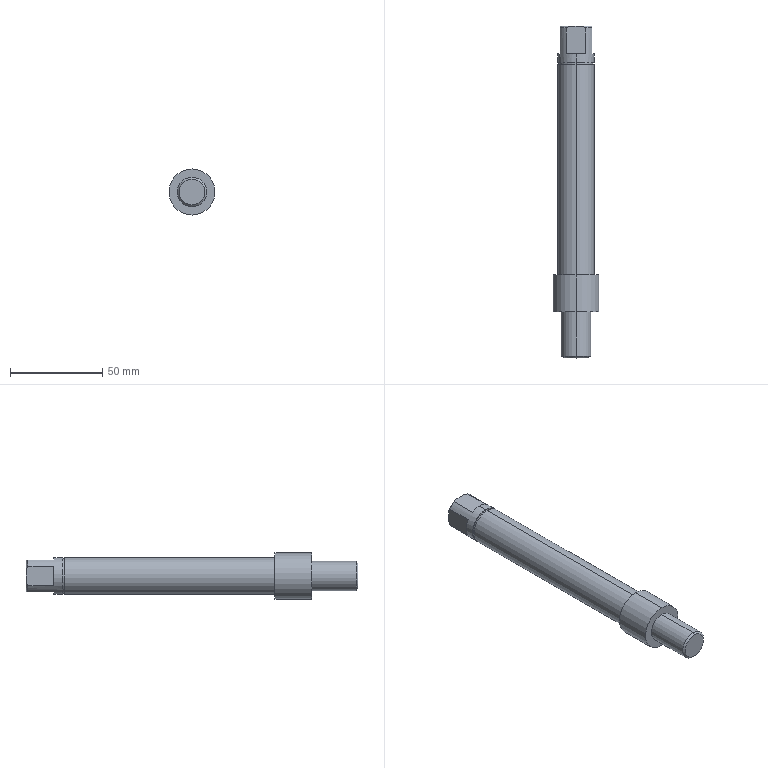Part | SolidWorks | features ICE 3, Chamfer 1, RevCut 1, Revolution 1 | 1 solid | 30 faces | box 25 x 180 x 25 mm | volume 56541 mm3 | plane 14 | cylinder 10 | cone 6 | commonest cylinder face diameters 20 x4 16 x2 19 x2 25 x2
STEP:
#1=CARTESIAN_POINT('',(0.,165.,10.));
#2=VERTEX_POINT('',#1);
#3=CARTESIAN_POINT('',(5.268,165.,8.5));
#4=VERTEX_POINT('',#3);
#5=CARTESIAN_POINT('',(0.,165.,0.));
#6=DIRECTION('',(0.,1.,0.));
#7=DIRECTION('',(0.,0.,-1.));
#8=AXIS2_PLACEMENT_3D('',#5,#6,#7);
#9=CIRCLE('',#8,10.);
#10=EDGE_CURVE('',#2,#4,#9,.T.);
#11=ORIENTED_EDGE('',*,*,#10,.F.);
#12=CARTESIAN_POINT('',(0.,160.2,10.));
#13=VERTEX_POINT('',#12);
#14=CARTESIAN_POINT('',(0.,0.,10.));
#15=DIRECTION('',(0.,-1.,0.));
#16=VECTOR('',#15,1000.);
#17=LINE('',#14,#16);
#18=EDGE_CURVE('',#2,#13,#17,.T.);
#19=ORIENTED_EDGE('',*,*,#18,.T.);
#20=CARTESIAN_POINT('',(0.,160.2,-10.));
#21=VERTEX_POINT('',#20);
#22=CARTESIAN_POINT('',(0.,160.2,0.));
#23=DIRECTION('',(0.,-1.,0.));
#24=DIRECTION('',(0.,0.,1.));
#25=AXIS2_PLACEMENT_3D('',#22,#23,#24);
#26=CIRCLE('',#25,10.);
#27=EDGE_CURVE('',#21,#13,#26,.T.);
#28=ORIENTED_EDGE('',*,*,#27,.F.);
#29=CARTESIAN_POINT('',(0.,165.,-10.));
#30=VERTEX_POINT('',#29);
#31=CARTESIAN_POINT('',(0.,0.,-10.));
#32=DIRECTION('',(0.,-1.,0.));
#33=VECTOR('',#32,1000.);
#34=LINE('',#31,#33);
#35=EDGE_CURVE('',#30,#21,#34,.T.);
#36=ORIENTED_EDGE('',*,*,#35,.F.);
#37=CARTESIAN_POINT('',(5.268,165.,-8.5));
#38=VERTEX_POINT('',#37);
#39=CARTESIAN_POINT('',(0.,165.,0.));
#40=DIRECTION('',(0.,1.,0.));
#41=DIRECTION('',(0.,0.,-1.));
#42=AXIS2_PLACEMENT_3D('',#39,#40,#41);
#43=CIRCLE('',#42,10.);
#44=EDGE_CURVE('',#38,#30,#43,.T.);
#45=ORIENTED_EDGE('',*,*,#44,.F.);
#46=CARTESIAN_POINT('',(5.268,179.,-8.5));
#47=VERTEX_POINT('',#46);
#48=CARTESIAN_POINT('',(5.268,0.,-8.5));
#49=DIRECTION('',(0.,-1.,0.));
#50=VECTOR('',#49,1000.);
#51=LINE('',#48,#50);
#52=EDGE_CURVE('',#47,#38,#51,.T.);
#53=ORIENTED_EDGE('',*,*,#52,.F.);
#54=CARTESIAN_POINT('',(8.5,179.,-5.268));
#55=VERTEX_POINT('',#54);
#56=CARTESIAN_POINT('',(0.,179.,0.));
#57=DIRECTION('',(0.,-1.,0.));
#58=DIRECTION('',(0.,0.,1.));
#59=AXIS2_PLACEMENT_3D('',#56,#57,#58);
#60=CIRCLE('',#59,10.);
#61=EDGE_CURVE('',#47,#55,#60,.T.);
#62=ORIENTED_EDGE('',*,*,#61,.T.);
#63=CARTESIAN_POINT('',(8.5,165.,-5.268));
#64=VERTEX_POINT('',#63);
#65=CARTESIAN_POINT('',(8.5,0.,-5.268));
#66=DIRECTION('',(0.,1.,0.));
#67=VECTOR('',#66,1000.);
#68=LINE('',#65,#67);
#69=EDGE_CURVE('',#64,#55,#68,.T.);
#70=ORIENTED_EDGE('',*,*,#69,.F.);
#71=CARTESIAN_POINT('',(8.5,165.,5.268));
#72=VERTEX_POINT('',#71);
#73=CARTESIAN_POINT('',(0.,165.,0.));
#74=DIRECTION('',(0.,1.,0.));
#75=DIRECTION('',(0.,0.,-1.));
#76=AXIS2_PLACEMENT_3D('',#73,#74,#75);
#77=CIRCLE('',#76,10.);
#78=EDGE_CURVE('',#72,#64,#77,.T.);
#79=ORIENTED_EDGE('',*,*,#78,.F.);
#80=CARTESIAN_POINT('',(8.5,179.,5.268));
#81=VERTEX_POINT('',#80);
#82=CARTESIAN_POINT('',(8.5,0.,5.268));
#83=DIRECTION('',(0.,-1.,0.));
#84=VECTOR('',#83,1000.);
#85=LINE('',#82,#84);
#86=EDGE_CURVE('',#81,#72,#85,.T.);
#87=ORIENTED_EDGE('',*,*,#86,.F.);
#88=CARTESIAN_POINT('',(5.268,179.,8.5));
#89=VERTEX_POINT('',#88);
#90=CARTESIAN_POINT('',(0.,179.,0.));
#91=DIRECTION('',(0.,-1.,0.));
#92=DIRECTION('',(0.,0.,1.));
#93=AXIS2_PLACEMENT_3D('',#90,#91,#92);
#94=CIRCLE('',#93,10.);
#95=EDGE_CURVE('',#81,#89,#94,.T.);
#96=ORIENTED_EDGE('',*,*,#95,.T.);
#97=CARTESIAN_POINT('',(5.268,0.,8.5));
#98=DIRECTION('',(0.,1.,0.));
#99=VECTOR('',#98,1000.);
#100=LINE('',#97,#99);
#101=EDGE_CURVE('',#4,#89,#100,.T.);
#102=ORIENTED_EDGE('',*,*,#101,.F.);
#103=EDGE_LOOP('',(#11,#19,#28,#36,#45,#53,#62,#70,#79,#87,#96,#102));
#104=FACE_OUTER_BOUND('',#103,.T.);
#105=CARTESIAN_POINT('',(0.,0.,0.));
#106=DIRECTION('',(0.,-1.,0.));
#107=DIRECTION('',(0.,0.,-1.));
#108=AXIS2_PLACEMENT_3D('',#105,#106,#107);
#109=CYLINDRICAL_SURFACE('',#108,10.);
#110=ADVANCED_FACE('',(#104),#109,.T.);
#111=CARTESIAN_POINT('',(0.,159.,9.5));
#112=VERTEX_POINT('',#111);
#113=CARTESIAN_POINT('',(0.,159.,-9.5));
#114=VERTEX_POINT('',#113);
#115=CARTESIAN_POINT('',(0.,159.,0.));
#116=DIRECTION('',(0.,1.,0.));
#117=DIRECTION('',(0.,0.,1.));
#118=AXIS2_PLACEMENT_3D('',#115,#116,#117);
#119=CIRCLE('',#118,9.5);
#120=EDGE_CURVE('',#112,#114,#119,.T.);
#121=ORIENTED_EDGE('',*,*,#120,.T.);
#122=CARTESIAN_POINT('',(0.,160.2,-9.5));
#123=VERTEX_POINT('',#122);
#124=CARTESIAN_POINT('',(0.,180.,-9.5));
#125=DIRECTION('',(0.,1.,0.));
#126=VECTOR('',#125,1000.);
#127=LINE('',#124,#126);
#128=EDGE_CURVE('',#114,#123,#127,.T.);
#129=ORIENTED_EDGE('',*,*,#128,.T.);
#130=CARTESIAN_POINT('',(0.,160.2,9.5));
#131=VERTEX_POINT('',#130);
#132=CARTESIAN_POINT('',(0.,160.2,0.));
#133=DIRECTION('',(0.,1.,0.));
#134=DIRECTION('',(0.,0.,1.));
#135=AXIS2_PLACEMENT_3D('',#132,#133,#134);
#136=CIRCLE('',#135,9.5);
#137=EDGE_CURVE('',#131,#123,#136,.T.);
#138=ORIENTED_EDGE('',*,*,#137,.F.);
#139=CARTESIAN_POINT('',(0.,180.,9.5));
#140=DIRECTION('',(0.,1.,0.));
#141=VECTOR('',#140,1000.);
#142=LINE('',#139,#141);
#143=EDGE_CURVE('',#112,#131,#142,.T.);
#144=ORIENTED_EDGE('',*,*,#143,.F.);
#145=EDGE_LOOP('',(#121,#129,#138,#144));
#146=FACE_OUTER_BOUND('',#145,.T.);
#147=CARTESIAN_POINT('',(0.,180.,0.));
#148=DIRECTION('',(0.,1.,0.));
#149=DIRECTION('',(0.,0.,1.));
#150=AXIS2_PLACEMENT_3D('',#147,#148,#149);
#151=CYLINDRICAL_SURFACE('',#150,9.5);
#152=ADVANCED_FACE('',(#146),#151,.T.);
#153=CARTESIAN_POINT('',(0.,0.,-7.));
#154=VERTEX_POINT('',#153);
#155=CARTESIAN_POINT('',(0.,0.,7.));
#156=VERTEX_POINT('',#155);
#157=CARTESIAN_POINT('',(0.,0.,0.));
#158=DIRECTION('',(0.,-1.,0.));
#159=DIRECTION('',(0.,0.,-1.));
#160=AXIS2_PLACEMENT_3D('',#157,#158,#159);
#161=CIRCLE('',#160,7.);
#162=EDGE_CURVE('',#154,#156,#161,.T.);
#163=ORIENTED_EDGE('',*,*,#162,.F.);
#164=CARTESIAN_POINT('',(0.,1.,-8.));
#165=VERTEX_POINT('',#164);
#166=CARTESIAN_POINT('',(0.,0.,-7.));
#167=DIRECTION('',(0.,0.7071,-0.7071));
#168=VECTOR('',#167,1000.);
#169=LINE('',#166,#168);
#170=EDGE_CURVE('',#154,#165,#169,.T.);
#171=ORIENTED_EDGE('',*,*,#170,.T.);
#172=CARTESIAN_POINT('',(0.,1.,8.));
#173=VERTEX_POINT('',#172);
#174=CARTESIAN_POINT('',(0.,1.,0.));
#175=DIRECTION('',(0.,1.,0.));
#176=DIRECTION('',(0.,0.,-1.));
#177=AXIS2_PLACEMENT_3D('',#174,#175,#176);
#178=CIRCLE('',#177,8.);
#179=EDGE_CURVE('',#173,#165,#178,.T.);
#180=ORIENTED_EDGE('',*,*,#179,.F.);
#181=CARTESIAN_POINT('',(0.,0.,7.));
#182=DIRECTION('',(0.,0.7071,0.7071));
#183=VECTOR('',#182,1000.);
#184=LINE('',#181,#183);
#185=EDGE_CURVE('',#156,#173,#184,.T.);
#186=ORIENTED_EDGE('',*,*,#185,.F.);
#187=EDGE_LOOP('',(#163,#171,#180,#186));
#188=FACE_OUTER_BOUND('',#187,.T.);
#189=CARTESIAN_POINT('',(0.,0.,0.));
#190=DIRECTION('',(0.,1.,0.));
#191=DIRECTION('',(0.,0.,1.));
#192=AXIS2_PLACEMENT_3D('',#189,#190,#191);
#193=CONICAL_SURFACE('',#192,7.,0.7854);
#194=ADVANCED_FACE('',(#188),#193,.T.);
#195=CARTESIAN_POINT('',(0.,25.,-8.));
#196=VERTEX_POINT('',#195);
#197=CARTESIAN_POINT('',(0.,25.,8.));
#198=VERTEX_POINT('',#197);
#199=CARTESIAN_POINT('',(0.,25.,0.));
#200=DIRECTION('',(0.,-1.,0.));
#201=DIRECTION('',(0.,0.,-1.));
#202=AXIS2_PLACEMENT_3D('',#199,#200,#201);
#203=CIRCLE('',#202,8.);
#204=EDGE_CURVE('',#196,#198,#203,.T.);
#205=ORIENTED_EDGE('',*,*,#204,.T.);
#206=CARTESIAN_POINT('',(0.,0.,8.));
#207=DIRECTION('',(0.,-1.,0.));
#208=VECTOR('',#207,1000.);
#209=LINE('',#206,#208);
#210=EDGE_CURVE('',#198,#173,#209,.T.);
#211=ORIENTED_EDGE('',*,*,#210,.T.);
#212=ORIENTED_EDGE('',*,*,#179,.T.);
#213=CARTESIAN_POINT('',(0.,0.,-8.));
#214=DIRECTION('',(0.,-1.,0.));
#215=VECTOR('',#214,1000.);
#216=LINE('',#213,#215);
#217=EDGE_CURVE('',#196,#165,#216,.T.);
#218=ORIENTED_EDGE('',*,*,#217,.F.);
#219=EDGE_LOOP('',(#205,#211,#212,#218));
#220=FACE_OUTER_BOUND('',#219,.T.);
#221=CARTESIAN_POINT('',(0.,0.,0.));
#222=DIRECTION('',(0.,-1.,0.));
#223=DIRECTION('',(0.,0.,-1.));
#224=AXIS2_PLACEMENT_3D('',#221,#222,#223);
#225=CYLINDRICAL_SURFACE('',#224,8.);
#226=ADVANCED_FACE('',(#220),#225,.T.);
#227=CARTESIAN_POINT('',(0.,45.,-12.5));
#228=VERTEX_POINT('',#227);
#229=CARTESIAN_POINT('',(0.,45.,12.5));
#230=VERTEX_POINT('',#229);
#231=CARTESIAN_POINT('',(0.,45.,0.));
#232=DIRECTION('',(0.,-1.,0.));
#233=DIRECTION('',(0.,0.,-1.));
#234=AXIS2_PLACEMENT_3D('',#231,#232,#233);
#235=CIRCLE('',#234,12.5);
#236=EDGE_CURVE('',#228,#230,#235,.T.);
#237=ORIENTED_EDGE('',*,*,#236,.T.);
#238=CARTESIAN_POINT('',(0.,25.,12.5));
#239=VERTEX_POINT('',#238);
#240=CARTESIAN_POINT('',(0.,0.,12.5));
#241=DIRECTION('',(0.,-1.,0.));
#242=VECTOR('',#241,1000.);
#243=LINE('',#240,#242);
#244=EDGE_CURVE('',#230,#239,#243,.T.);
#245=ORIENTED_EDGE('',*,*,#244,.T.);
#246=CARTESIAN_POINT('',(0.,25.,-12.5));
#247=VERTEX_POINT('',#246);
#248=CARTESIAN_POINT('',(0.,25.,0.));
#249=DIRECTION('',(0.,-1.,0.));
#250=DIRECTION('',(0.,0.,-1.));
#251=AXIS2_PLACEMENT_3D('',#248,#249,#250);
#252=CIRCLE('',#251,12.5);
#253=EDGE_CURVE('',#247,#239,#252,.T.);
#254=ORIENTED_EDGE('',*,*,#253,.F.);
#255=CARTESIAN_POINT('',(0.,0.,-12.5));
#256=DIRECTION('',(0.,-1.,0.));
#257=VECTOR('',#256,1000.);
#258=LINE('',#255,#257);
#259=EDGE_CURVE('',#228,#247,#258,.T.);
#260=ORIENTED_EDGE('',*,*,#259,.F.);
#261=EDGE_LOOP('',(#237,#245,#254,#260));
#262=FACE_OUTER_BOUND('',#261,.T.);
#263=CARTESIAN_POINT('',(0.,0.,0.));
#264=DIRECTION('',(0.,-1.,0.));
#265=DIRECTION('',(0.,0.,-1.));
#266=AXIS2_PLACEMENT_3D('',#263,#264,#265);
#267=CYLINDRICAL_SURFACE('',#266,12.5);
#268=ADVANCED_FACE('',(#262),#267,.T.);
#269=CARTESIAN_POINT('',(0.,159.,10.));
#270=VERTEX_POINT('',#269);
#271=CARTESIAN_POINT('',(0.,159.,-10.));
#272=VERTEX_POINT('',#271);
#273=CARTESIAN_POINT('',(0.,159.,0.));
#274=DIRECTION('',(0.,1.,0.));
#275=DIRECTION('',(0.,0.,-1.));
#276=AXIS2_PLACEMENT_3D('',#273,#274,#275);
#277=CIRCLE('',#276,10.);
#278=EDGE_CURVE('',#270,#272,#277,.T.);
#279=ORIENTED_EDGE('',*,*,#278,.F.);
#280=CARTESIAN_POINT('',(0.,45.,10.));
#281=VERTEX_POINT('',#280);
#282=CARTESIAN_POINT('',(0.,0.,10.));
#283=DIRECTION('',(0.,-1.,0.));
#284=VECTOR('',#283,1000.);
#285=LINE('',#282,#284);
#286=EDGE_CURVE('',#270,#281,#285,.T.);
#287=ORIENTED_EDGE('',*,*,#286,.T.);
#288=CARTESIAN_POINT('',(0.,45.,-10.));
#289=VERTEX_POINT('',#288);
#290=CARTESIAN_POINT('',(0.,45.,0.));
#291=DIRECTION('',(0.,-1.,0.));
#292=DIRECTION('',(0.,0.,-1.));
#293=AXIS2_PLACEMENT_3D('',#290,#291,#292);
#294=CIRCLE('',#293,10.);
#295=EDGE_CURVE('',#289,#281,#294,.T.);
#296=ORIENTED_EDGE('',*,*,#295,.F.);
#297=CARTESIAN_POINT('',(0.,0.,-10.));
#298=DIRECTION('',(0.,-1.,0.));
#299=VECTOR('',#298,1000.);
#300=LINE('',#297,#299);
#301=EDGE_CURVE('',#272,#289,#300,.T.);
#302=ORIENTED_EDGE('',*,*,#301,.F.);
#303=EDGE_LOOP('',(#279,#287,#296,#302));
#304=FACE_OUTER_BOUND('',#303,.T.);
#305=CARTESIAN_POINT('',(0.,0.,0.));
#306=DIRECTION('',(0.,-1.,0.));
#307=DIRECTION('',(0.,0.,-1.));
#308=AXIS2_PLACEMENT_3D('',#305,#306,#307);
#309=CYLINDRICAL_SURFACE('',#308,10.);
#310=ADVANCED_FACE('',(#304),#309,.T.);
#311=CARTESIAN_POINT('',(2.958,180.,8.5));
#312=VERTEX_POINT('',#311);
#313=CARTESIAN_POINT('',(5.268,179.,8.5));
#314=CARTESIAN_POINT('',(4.522,179.393,8.5));
#315=CARTESIAN_POINT('',(3.757,179.738,8.5));
#316=CARTESIAN_POINT('',(2.958,180.,8.5));
#317=B_SPLINE_CURVE_WITH_KNOTS('',3,(#313,#314,#315,#316),.UNSPECIFIED.,.F.,.F.,(4,4),(0.01663,0.01916),.UNSPECIFIED.);
#318=EDGE_CURVE('',#89,#312,#317,.T.);
#319=ORIENTED_EDGE('',*,*,#318,.F.);
#320=ORIENTED_EDGE('',*,*,#95,.F.);
#321=CARTESIAN_POINT('',(8.5,180.,2.958));
#322=VERTEX_POINT('',#321);
#323=CARTESIAN_POINT('',(8.5,180.,2.958));
#324=CARTESIAN_POINT('',(8.5,179.868,3.36));
#325=CARTESIAN_POINT('',(8.5,179.714,3.755));
#326=CARTESIAN_POINT('',(8.5,179.378,4.523));
#327=CARTESIAN_POINT('',(8.5,179.194,4.899));
#328=CARTESIAN_POINT('',(8.5,179.,5.268));
#329=B_SPLINE_CURVE_WITH_KNOTS('',3,(#323,#324,#325,#326,#327,#328),.UNSPECIFIED.,.F.,.F.,(4,2,4),(0.02784,0.02911,0.03037),.UNSPECIFIED.);
#330=EDGE_CURVE('',#322,#81,#329,.T.);
#331=ORIENTED_EDGE('',*,*,#330,.F.);
#332=CARTESIAN_POINT('',(0.,180.,0.));
#333=DIRECTION('',(0.,1.,0.));
#334=DIRECTION('',(0.,0.,1.));
#335=AXIS2_PLACEMENT_3D('',#332,#333,#334);
#336=CIRCLE('',#335,9.);
#337=EDGE_CURVE('',#312,#322,#336,.T.);
#338=ORIENTED_EDGE('',*,*,#337,.F.);
#339=EDGE_LOOP('',(#319,#320,#331,#338));
#340=FACE_OUTER_BOUND('',#339,.T.);
#341=CARTESIAN_POINT('',(0.,179.,0.));
#342=DIRECTION('',(0.,-1.,0.));
#343=DIRECTION('',(0.,0.,-1.));
#344=AXIS2_PLACEMENT_3D('',#341,#342,#343);
#345=CONICAL_SURFACE('',#344,10.,0.7854);
#346=ADVANCED_FACE('',(#340),#345,.T.);
#347=CARTESIAN_POINT('',(-5.268,179.,-8.5));
#348=VERTEX_POINT('',#347);
#349=CARTESIAN_POINT('',(-2.958,180.,-8.5));
#350=VERTEX_POINT('',#349);
#351=CARTESIAN_POINT('',(-5.268,179.,-8.5));
#352=CARTESIAN_POINT('',(-4.522,179.393,-8.5));
#353=CARTESIAN_POINT('',(-3.757,179.738,-8.5));
#354=CARTESIAN_POINT('',(-2.958,180.,-8.5));
#355=B_SPLINE_CURVE_WITH_KNOTS('',3,(#351,#352,#353,#354),.UNSPECIFIED.,.F.,.F.,(4,4),(0.01663,0.01916),.UNSPECIFIED.);
#356=EDGE_CURVE('',#348,#350,#355,.T.);
#357=ORIENTED_EDGE('',*,*,#356,.F.);
#358=CARTESIAN_POINT('',(-8.5,179.,-5.268));
#359=VERTEX_POINT('',#358);
#360=CARTESIAN_POINT('',(0.,179.,0.));
#361=DIRECTION('',(0.,-1.,0.));
#362=DIRECTION('',(0.,0.,1.));
#363=AXIS2_PLACEMENT_3D('',#360,#361,#362);
#364=CIRCLE('',#363,10.);
#365=EDGE_CURVE('',#359,#348,#364,.T.);
#366=ORIENTED_EDGE('',*,*,#365,.F.);
#367=CARTESIAN_POINT('',(-8.5,180.,-2.958));
#368=VERTEX_POINT('',#367);
#369=CARTESIAN_POINT('',(-8.5,180.,-2.958));
#370=CARTESIAN_POINT('',(-8.5,179.868,-3.36));
#371=CARTESIAN_POINT('',(-8.5,179.714,-3.755));
#372=CARTESIAN_POINT('',(-8.5,179.378,-4.523));
#373=CARTESIAN_POINT('',(-8.5,179.194,-4.899));
#374=CARTESIAN_POINT('',(-8.5,179.,-5.268));
#375=B_SPLINE_CURVE_WITH_KNOTS('',3,(#369,#370,#371,#372,#373,#374),.UNSPECIFIED.,.F.,.F.,(4,2,4),(0.02784,0.02911,0.03037),.UNSPECIFIED.);
#376=EDGE_CURVE('',#368,#359,#375,.T.);
#377=ORIENTED_EDGE('',*,*,#376,.F.);
#378=CARTESIAN_POINT('',(0.,180.,0.));
#379=DIRECTION('',(0.,1.,0.));
#380=DIRECTION('',(0.,0.,1.));
#381=AXIS2_PLACEMENT_3D('',#378,#379,#380);
#382=CIRCLE('',#381,9.);
#383=EDGE_CURVE('',#350,#368,#382,.T.);
#384=ORIENTED_EDGE('',*,*,#383,.F.);
#385=EDGE_LOOP('',(#357,#366,#377,#384));
#386=FACE_OUTER_BOUND('',#385,.T.);
#387=CARTESIAN_POINT('',(0.,179.,0.));
#388=DIRECTION('',(0.,-1.,0.));
#389=DIRECTION('',(0.,0.,-1.));
#390=AXIS2_PLACEMENT_3D('',#387,#388,#389);
#391=CONICAL_SURFACE('',#390,10.,0.7854);
#392=ADVANCED_FACE('',(#386),#391,.T.);
#393=CARTESIAN_POINT('',(-2.958,180.,8.5));
#394=VERTEX_POINT('',#393);
#395=CARTESIAN_POINT('',(-5.268,179.,8.5));
#396=VERTEX_POINT('',#395);
#397=CARTESIAN_POINT('',(-2.958,180.,8.5));
#398=CARTESIAN_POINT('',(-3.357,179.869,8.5));
#399=CARTESIAN_POINT('',(-3.752,179.715,8.5));
#400=CARTESIAN_POINT('',(-4.523,179.378,8.5));
#401=CARTESIAN_POINT('',(-4.899,179.194,8.5));
#402=CARTESIAN_POINT('',(-5.268,179.,8.5));
#403=B_SPLINE_CURVE_WITH_KNOTS('',3,(#397,#398,#399,#400,#401,#402),.UNSPECIFIED.,.F.,.F.,(4,2,4),(0.02518,0.02643,0.02769),.UNSPECIFIED.);
#404=EDGE_CURVE('',#394,#396,#403,.T.);
#405=ORIENTED_EDGE('',*,*,#404,.F.);
#406=CARTESIAN_POINT('',(-8.5,180.,2.958));
#407=VERTEX_POINT('',#406);
#408=CARTESIAN_POINT('',(0.,180.,0.));
#409=DIRECTION('',(0.,1.,0.));
#410=DIRECTION('',(0.,0.,1.));
#411=AXIS2_PLACEMENT_3D('',#408,#409,#410);
#412=CIRCLE('',#411,9.);
#413=EDGE_CURVE('',#407,#394,#412,.T.);
#414=ORIENTED_EDGE('',*,*,#413,.F.);
#415=CARTESIAN_POINT('',(-8.5,179.,5.268));
#416=VERTEX_POINT('',#415);
#417=CARTESIAN_POINT('',(-8.5,179.,5.268));
#418=CARTESIAN_POINT('',(-8.5,179.391,4.525));
#419=CARTESIAN_POINT('',(-8.5,179.736,3.761));
#420=CARTESIAN_POINT('',(-8.5,180.,2.958));
#421=B_SPLINE_CURVE_WITH_KNOTS('',3,(#417,#418,#419,#420),.UNSPECIFIED.,.F.,.F.,(4,4),(0.01929,0.02181),.UNSPECIFIED.);
#422=EDGE_CURVE('',#416,#407,#421,.T.);
#423=ORIENTED_EDGE('',*,*,#422,.F.);
#424=CARTESIAN_POINT('',(0.,179.,0.));
#425=DIRECTION('',(0.,-1.,0.));
#426=DIRECTION('',(0.,0.,1.));
#427=AXIS2_PLACEMENT_3D('',#424,#425,#426);
#428=CIRCLE('',#427,10.);
#429=EDGE_CURVE('',#396,#416,#428,.T.);
#430=ORIENTED_EDGE('',*,*,#429,.F.);
#431=EDGE_LOOP('',(#405,#414,#423,#430));
#432=FACE_OUTER_BOUND('',#431,.T.);
#433=CARTESIAN_POINT('',(0.,179.,0.));
#434=DIRECTION('',(0.,-1.,0.));
#435=DIRECTION('',(0.,0.,-1.));
#436=AXIS2_PLACEMENT_3D('',#433,#434,#435);
#437=CONICAL_SURFACE('',#436,10.,0.7854);
#438=ADVANCED_FACE('',(#432),#437,.T.);
#439=ORIENTED_EDGE('',*,*,#286,.F.);
#440=CARTESIAN_POINT('',(0.,159.,0.));
#441=DIRECTION('',(0.,1.,0.));
#442=DIRECTION('',(0.,0.,-1.));
#443=AXIS2_PLACEMENT_3D('',#440,#441,#442);
#444=CIRCLE('',#443,10.);
#445=EDGE_CURVE('',#272,#270,#444,.T.);
#446=ORIENTED_EDGE('',*,*,#445,.F.);
#447=ORIENTED_EDGE('',*,*,#301,.T.);
#448=CARTESIAN_POINT('',(0.,45.,0.));
#449=DIRECTION('',(0.,-1.,0.));
#450=DIRECTION('',(0.,0.,-1.));
#451=AXIS2_PLACEMENT_3D('',#448,#449,#450);
#452=CIRCLE('',#451,10.);
#453=EDGE_CURVE('',#281,#289,#452,.T.);
#454=ORIENTED_EDGE('',*,*,#453,.F.);
#455=EDGE_LOOP('',(#439,#446,#447,#454));
#456=FACE_OUTER_BOUND('',#455,.T.);
#457=CARTESIAN_POINT('',(0.,0.,0.));
#458=DIRECTION('',(0.,-1.,0.));
#459=DIRECTION('',(0.,0.,-1.));
#460=AXIS2_PLACEMENT_3D('',#457,#458,#459);
#461=CYLINDRICAL_SURFACE('',#460,10.);
#462=ADVANCED_FACE('',(#456),#461,.T.);
#463=CARTESIAN_POINT('',(0.,0.,0.));
#464=DIRECTION('',(0.,-1.,0.));
#465=DIRECTION('',(0.,0.,-1.));
#466=AXIS2_PLACEMENT_3D('',#463,#464,#465);
#467=CIRCLE('',#466,7.);
#468=EDGE_CURVE('',#156,#154,#467,.T.);
#469=ORIENTED_EDGE('',*,*,#468,.T.);
#470=ORIENTED_EDGE('',*,*,#162,.T.);
#471=EDGE_LOOP('',(#469,#470));
#472=FACE_OUTER_BOUND('',#471,.T.);
#473=CARTESIAN_POINT('',(8.,0.,0.));
#474=DIRECTION('',(0.,-1.,0.));
#475=DIRECTION('',(0.,0.,-1.));
#476=AXIS2_PLACEMENT_3D('',#473,#474,#475);
#477=PLANE('',#476);
#478=ADVANCED_FACE('',(#472),#477,.T.);
#479=ORIENTED_EDGE('',*,*,#295,.T.);
#480=ORIENTED_EDGE('',*,*,#453,.T.);
#481=EDGE_LOOP('',(#479,#480));
#482=FACE_BOUND('',#481,.T.);
#483=ORIENTED_EDGE('',*,*,#236,.F.);
#484=CARTESIAN_POINT('',(0.,45.,0.));
#485=DIRECTION('',(0.,-1.,0.));
#486=DIRECTION('',(0.,0.,-1.));
#487=AXIS2_PLACEMENT_3D('',#484,#485,#486);
#488=CIRCLE('',#487,12.5);
#489=EDGE_CURVE('',#230,#228,#488,.T.);
#490=ORIENTED_EDGE('',*,*,#489,.F.);
#491=EDGE_LOOP('',(#483,#490));
#492=FACE_OUTER_BOUND('',#491,.T.);
#493=CARTESIAN_POINT('',(10.,45.,0.));
#494=DIRECTION('',(0.,1.,0.));
#495=DIRECTION('',(0.,0.,1.));
#496=AXIS2_PLACEMENT_3D('',#493,#494,#495);
#497=PLANE('',#496);
#498=ADVANCED_FACE('',(#482,#492),#497,.T.);
#499=ORIENTED_EDGE('',*,*,#244,.F.);
#500=ORIENTED_EDGE('',*,*,#489,.T.);
#501=ORIENTED_EDGE('',*,*,#259,.T.);
#502=CARTESIAN_POINT('',(0.,25.,0.));
#503=DIRECTION('',(0.,-1.,0.));
#504=DIRECTION('',(0.,0.,-1.));
#505=AXIS2_PLACEMENT_3D('',#502,#503,#504);
#506=CIRCLE('',#505,12.5);
#507=EDGE_CURVE('',#239,#247,#506,.T.);
#508=ORIENTED_EDGE('',*,*,#507,.F.);
#509=EDGE_LOOP('',(#499,#500,#501,#508));
#510=FACE_OUTER_BOUND('',#509,.T.);
#511=CARTESIAN_POINT('',(0.,0.,0.));
#512=DIRECTION('',(0.,-1.,0.));
#513=DIRECTION('',(0.,0.,-1.));
#514=AXIS2_PLACEMENT_3D('',#511,#512,#513);
#515=CYLINDRICAL_SURFACE('',#514,12.5);
#516=ADVANCED_FACE('',(#510),#515,.T.);
#517=ORIENTED_EDGE('',*,*,#253,.T.);
#518=ORIENTED_EDGE('',*,*,#507,.T.);
#519=EDGE_LOOP('',(#517,#518));
#520=FACE_OUTER_BOUND('',#519,.T.);
#521=ORIENTED_EDGE('',*,*,#204,.F.);
#522=CARTESIAN_POINT('',(0.,25.,0.));
#523=DIRECTION('',(0.,-1.,0.));
#524=DIRECTION('',(0.,0.,-1.));
#525=AXIS2_PLACEMENT_3D('',#522,#523,#524);
#526=CIRCLE('',#525,8.);
#527=EDGE_CURVE('',#198,#196,#526,.T.);
#528=ORIENTED_EDGE('',*,*,#527,.F.);
#529=EDGE_LOOP('',(#521,#528));
#530=FACE_BOUND('',#529,.T.);
#531=CARTESIAN_POINT('',(8.,25.,0.));
#532=DIRECTION('',(0.,-1.,0.));
#533=DIRECTION('',(0.,0.,-1.));
#534=AXIS2_PLACEMENT_3D('',#531,#532,#533);
#535=PLANE('',#534);
#536=ADVANCED_FACE('',(#520,#530),#535,.T.);
#537=ORIENTED_EDGE('',*,*,#210,.F.);
#538=ORIENTED_EDGE('',*,*,#527,.T.);
#539=ORIENTED_EDGE('',*,*,#217,.T.);
#540=CARTESIAN_POINT('',(0.,1.,0.));
#541=DIRECTION('',(0.,1.,0.));
#542=DIRECTION('',(0.,0.,-1.));
#543=AXIS2_PLACEMENT_3D('',#540,#541,#542);
#544=CIRCLE('',#543,8.);
#545=EDGE_CURVE('',#165,#173,#544,.T.);
#546=ORIENTED_EDGE('',*,*,#545,.T.);
#547=EDGE_LOOP('',(#537,#538,#539,#546));
#548=FACE_OUTER_BOUND('',#547,.T.);
#549=CARTESIAN_POINT('',(0.,0.,0.));
#550=DIRECTION('',(0.,-1.,0.));
#551=DIRECTION('',(0.,0.,-1.));
#552=AXIS2_PLACEMENT_3D('',#549,#550,#551);
#553=CYLINDRICAL_SURFACE('',#552,8.);
#554=ADVANCED_FACE('',(#548),#553,.T.);
#555=ORIENTED_EDGE('',*,*,#170,.F.);
#556=ORIENTED_EDGE('',*,*,#468,.F.);
#557=ORIENTED_EDGE('',*,*,#185,.T.);
#558=ORIENTED_EDGE('',*,*,#545,.F.);
#559=EDGE_LOOP('',(#555,#556,#557,#558));
#560=FACE_OUTER_BOUND('',#559,.T.);
#561=CARTESIAN_POINT('',(0.,0.,0.));
#562=DIRECTION('',(0.,1.,0.));
#563=DIRECTION('',(0.,0.,1.));
#564=AXIS2_PLACEMENT_3D('',#561,#562,#563);
#565=CONICAL_SURFACE('',#564,7.,0.7854);
#566=ADVANCED_FACE('',(#560),#565,.T.);
#567=ORIENTED_EDGE('',*,*,#445,.T.);
#568=ORIENTED_EDGE('',*,*,#278,.T.);
#569=EDGE_LOOP('',(#567,#568));
#570=FACE_OUTER_BOUND('',#569,.T.);
#571=ORIENTED_EDGE('',*,*,#120,.F.);
#572=CARTESIAN_POINT('',(0.,159.,0.));
#573=DIRECTION('',(0.,1.,0.));
#574=DIRECTION('',(0.,0.,1.));
#575=AXIS2_PLACEMENT_3D('',#572,#573,#574);
#576=CIRCLE('',#575,9.5);
#577=EDGE_CURVE('',#114,#112,#576,.T.);
#578=ORIENTED_EDGE('',*,*,#577,.F.);
#579=EDGE_LOOP('',(#571,#578));
#580=FACE_BOUND('',#579,.T.);
#581=CARTESIAN_POINT('',(-15.299,159.,0.));
#582=DIRECTION('',(0.,-1.,0.));
#583=DIRECTION('',(0.,0.,-1.));
#584=AXIS2_PLACEMENT_3D('',#581,#582,#583);
#585=PLANE('',#584);
#586=ADVANCED_FACE('',(#570,#580),#585,.F.);
#587=ORIENTED_EDGE('',*,*,#128,.F.);
#588=ORIENTED_EDGE('',*,*,#577,.T.);
#589=ORIENTED_EDGE('',*,*,#143,.T.);
#590=CARTESIAN_POINT('',(0.,160.2,0.));
#591=DIRECTION('',(0.,1.,0.));
#592=DIRECTION('',(0.,0.,1.));
#593=AXIS2_PLACEMENT_3D('',#590,#591,#592);
#594=CIRCLE('',#593,9.5);
#595=EDGE_CURVE('',#123,#131,#594,.T.);
#596=ORIENTED_EDGE('',*,*,#595,.F.);
#597=EDGE_LOOP('',(#587,#588,#589,#596));
#598=FACE_OUTER_BOUND('',#597,.T.);
#599=CARTESIAN_POINT('',(0.,180.,0.));
#600=DIRECTION('',(0.,1.,0.));
#601=DIRECTION('',(0.,0.,1.));
#602=AXIS2_PLACEMENT_3D('',#599,#600,#601);
#603=CYLINDRICAL_SURFACE('',#602,9.5);
#604=ADVANCED_FACE('',(#598),#603,.T.);
#605=ORIENTED_EDGE('',*,*,#27,.T.);
#606=CARTESIAN_POINT('',(0.,160.2,0.));
#607=DIRECTION('',(0.,-1.,0.));
#608=DIRECTION('',(0.,0.,1.));
#609=AXIS2_PLACEMENT_3D('',#606,#607,#608);
#610=CIRCLE('',#609,10.);
#611=EDGE_CURVE('',#13,#21,#610,.T.);
#612=ORIENTED_EDGE('',*,*,#611,.T.);
#613=EDGE_LOOP('',(#605,#612));
#614=FACE_OUTER_BOUND('',#613,.T.);
#615=ORIENTED_EDGE('',*,*,#137,.T.);
#616=ORIENTED_EDGE('',*,*,#595,.T.);
#617=EDGE_LOOP('',(#615,#616));
#618=FACE_BOUND('',#617,.T.);
#619=CARTESIAN_POINT('',(-15.299,160.2,0.));
#620=DIRECTION('',(0.,1.,0.));
#621=DIRECTION('',(0.,0.,1.));
#622=AXIS2_PLACEMENT_3D('',#619,#620,#621);
#623=PLANE('',#622);
#624=ADVANCED_FACE('',(#614,#618),#623,.F.);
#625=CARTESIAN_POINT('',(0.,180.,8.5));
#626=DIRECTION('',(-1.,0.,0.));
#627=VECTOR('',#626,1000.);
#628=LINE('',#625,#627);
#629=EDGE_CURVE('',#312,#394,#628,.T.);
#630=ORIENTED_EDGE('',*,*,#629,.F.);
#631=ORIENTED_EDGE('',*,*,#337,.T.);
#632=CARTESIAN_POINT('',(8.5,180.,-2.958));
#633=VERTEX_POINT('',#632);
#634=CARTESIAN_POINT('',(8.5,180.,0.));
#635=DIRECTION('',(0.,0.,1.));
#636=VECTOR('',#635,1000.);
#637=LINE('',#634,#636);
#638=EDGE_CURVE('',#633,#322,#637,.T.);
#639=ORIENTED_EDGE('',*,*,#638,.F.);
#640=CARTESIAN_POINT('',(2.958,180.,-8.5));
#641=VERTEX_POINT('',#640);
#642=CARTESIAN_POINT('',(0.,180.,0.));
#643=DIRECTION('',(0.,1.,0.));
#644=DIRECTION('',(0.,0.,1.));
#645=AXIS2_PLACEMENT_3D('',#642,#643,#644);
#646=CIRCLE('',#645,9.);
#647=EDGE_CURVE('',#633,#641,#646,.T.);
#648=ORIENTED_EDGE('',*,*,#647,.T.);
#649=CARTESIAN_POINT('',(0.,180.,-8.5));
#650=DIRECTION('',(1.,0.,0.));
#651=VECTOR('',#650,1000.);
#652=LINE('',#649,#651);
#653=EDGE_CURVE('',#350,#641,#652,.T.);
#654=ORIENTED_EDGE('',*,*,#653,.F.);
#655=ORIENTED_EDGE('',*,*,#383,.T.);
#656=CARTESIAN_POINT('',(-8.5,180.,0.));
#657=DIRECTION('',(0.,0.,-1.));
#658=VECTOR('',#657,1000.);
#659=LINE('',#656,#658);
#660=EDGE_CURVE('',#407,#368,#659,.T.);
#661=ORIENTED_EDGE('',*,*,#660,.F.);
#662=ORIENTED_EDGE('',*,*,#413,.T.);
#663=EDGE_LOOP('',(#630,#631,#639,#648,#654,#655,#661,#662));
#664=FACE_OUTER_BOUND('',#663,.T.);
#665=CARTESIAN_POINT('',(0.,180.,0.));
#666=DIRECTION('',(0.,1.,0.));
#667=DIRECTION('',(0.,0.,1.));
#668=AXIS2_PLACEMENT_3D('',#665,#666,#667);
#669=PLANE('',#668);
#670=ADVANCED_FACE('',(#664),#669,.T.);
#671=CARTESIAN_POINT('',(2.958,180.,-8.5));
#672=CARTESIAN_POINT('',(3.357,179.869,-8.5));
#673=CARTESIAN_POINT('',(3.752,179.715,-8.5));
#674=CARTESIAN_POINT('',(4.523,179.378,-8.5));
#675=CARTESIAN_POINT('',(4.899,179.194,-8.5));
#676=CARTESIAN_POINT('',(5.268,179.,-8.5));
#677=B_SPLINE_CURVE_WITH_KNOTS('',3,(#671,#672,#673,#674,#675,#676),.UNSPECIFIED.,.F.,.F.,(4,2,4),(0.02518,0.02643,0.02769),.UNSPECIFIED.);
#678=EDGE_CURVE('',#641,#47,#677,.T.);
#679=ORIENTED_EDGE('',*,*,#678,.F.);
#680=ORIENTED_EDGE('',*,*,#647,.F.);
#681=CARTESIAN_POINT('',(8.5,179.,-5.268));
#682=CARTESIAN_POINT('',(8.5,179.391,-4.525));
#683=CARTESIAN_POINT('',(8.5,179.736,-3.761));
#684=CARTESIAN_POINT('',(8.5,180.,-2.958));
#685=B_SPLINE_CURVE_WITH_KNOTS('',3,(#681,#682,#683,#684),.UNSPECIFIED.,.F.,.F.,(4,4),(0.01929,0.02181),.UNSPECIFIED.);
#686=EDGE_CURVE('',#55,#633,#685,.T.);
#687=ORIENTED_EDGE('',*,*,#686,.F.);
#688=ORIENTED_EDGE('',*,*,#61,.F.);
#689=EDGE_LOOP('',(#679,#680,#687,#688));
#690=FACE_OUTER_BOUND('',#689,.T.);
#691=CARTESIAN_POINT('',(0.,179.,0.));
#692=DIRECTION('',(0.,-1.,0.));
#693=DIRECTION('',(0.,0.,-1.));
#694=AXIS2_PLACEMENT_3D('',#691,#692,#693);
#695=CONICAL_SURFACE('',#694,10.,0.7854);
#696=ADVANCED_FACE('',(#690),#695,.T.);
#697=ORIENTED_EDGE('',*,*,#18,.F.);
#698=CARTESIAN_POINT('',(-5.268,165.,8.5));
#699=VERTEX_POINT('',#698);
#700=CARTESIAN_POINT('',(0.,165.,0.));
#701=DIRECTION('',(0.,1.,0.));
#702=DIRECTION('',(0.,0.,-1.));
#703=AXIS2_PLACEMENT_3D('',#700,#701,#702);
#704=CIRCLE('',#703,10.);
#705=EDGE_CURVE('',#699,#2,#704,.T.);
#706=ORIENTED_EDGE('',*,*,#705,.F.);
#707=CARTESIAN_POINT('',(-5.268,0.,8.5));
#708=DIRECTION('',(0.,-1.,0.));
#709=VECTOR('',#708,1000.);
#710=LINE('',#707,#709);
#711=EDGE_CURVE('',#396,#699,#710,.T.);
#712=ORIENTED_EDGE('',*,*,#711,.F.);
#713=ORIENTED_EDGE('',*,*,#429,.T.);
#714=CARTESIAN_POINT('',(-8.5,165.,5.268));
#715=VERTEX_POINT('',#714);
#716=CARTESIAN_POINT('',(-8.5,0.,5.268));
#717=DIRECTION('',(0.,1.,0.));
#718=VECTOR('',#717,1000.);
#719=LINE('',#716,#718);
#720=EDGE_CURVE('',#715,#416,#719,.T.);
#721=ORIENTED_EDGE('',*,*,#720,.F.);
#722=CARTESIAN_POINT('',(-8.5,165.,-5.268));
#723=VERTEX_POINT('',#722);
#724=CARTESIAN_POINT('',(0.,165.,0.));
#725=DIRECTION('',(0.,1.,0.));
#726=DIRECTION('',(0.,0.,-1.));
#727=AXIS2_PLACEMENT_3D('',#724,#725,#726);
#728=CIRCLE('',#727,10.);
#729=EDGE_CURVE('',#723,#715,#728,.T.);
#730=ORIENTED_EDGE('',*,*,#729,.F.);
#731=CARTESIAN_POINT('',(-8.5,0.,-5.268));
#732=DIRECTION('',(0.,-1.,0.));
#733=VECTOR('',#732,1000.);
#734=LINE('',#731,#733);
#735=EDGE_CURVE('',#359,#723,#734,.T.);
#736=ORIENTED_EDGE('',*,*,#735,.F.);
#737=ORIENTED_EDGE('',*,*,#365,.T.);
#738=CARTESIAN_POINT('',(-5.268,165.,-8.5));
#739=VERTEX_POINT('',#738);
#740=CARTESIAN_POINT('',(-5.268,0.,-8.5));
#741=DIRECTION('',(0.,1.,0.));
#742=VECTOR('',#741,1000.);
#743=LINE('',#740,#742);
#744=EDGE_CURVE('',#739,#348,#743,.T.);
#745=ORIENTED_EDGE('',*,*,#744,.F.);
#746=CARTESIAN_POINT('',(0.,165.,0.));
#747=DIRECTION('',(0.,1.,0.));
#748=DIRECTION('',(0.,0.,-1.));
#749=AXIS2_PLACEMENT_3D('',#746,#747,#748);
#750=CIRCLE('',#749,10.);
#751=EDGE_CURVE('',#30,#739,#750,.T.);
#752=ORIENTED_EDGE('',*,*,#751,.F.);
#753=ORIENTED_EDGE('',*,*,#35,.T.);
#754=ORIENTED_EDGE('',*,*,#611,.F.);
#755=EDGE_LOOP('',(#697,#706,#712,#713,#721,#730,#736,#737,#745,#752,#753,#754));
#756=FACE_OUTER_BOUND('',#755,.T.);
#757=CARTESIAN_POINT('',(0.,0.,0.));
#758=DIRECTION('',(0.,-1.,0.));
#759=DIRECTION('',(0.,0.,-1.));
#760=AXIS2_PLACEMENT_3D('',#757,#758,#759);
#761=CYLINDRICAL_SURFACE('',#760,10.);
#762=ADVANCED_FACE('',(#756),#761,.T.);
#763=ORIENTED_EDGE('',*,*,#78,.T.);
#764=CARTESIAN_POINT('',(8.5,165.,-12.5));
#765=DIRECTION('',(0.,0.,1.));
#766=VECTOR('',#765,1000.);
#767=LINE('',#764,#766);
#768=EDGE_CURVE('',#64,#72,#767,.T.);
#769=ORIENTED_EDGE('',*,*,#768,.T.);
#770=EDGE_LOOP('',(#763,#769));
#771=FACE_OUTER_BOUND('',#770,.T.);
#772=CARTESIAN_POINT('',(21.149,165.,-12.5));
#773=DIRECTION('',(0.,-1.,0.));
#774=DIRECTION('',(0.,0.,-1.));
#775=AXIS2_PLACEMENT_3D('',#772,#773,#774);
#776=PLANE('',#775);
#777=ADVANCED_FACE('',(#771),#776,.F.);
#778=ORIENTED_EDGE('',*,*,#69,.T.);
#779=ORIENTED_EDGE('',*,*,#686,.T.);
#780=ORIENTED_EDGE('',*,*,#638,.T.);
#781=ORIENTED_EDGE('',*,*,#330,.T.);
#782=ORIENTED_EDGE('',*,*,#86,.T.);
#783=ORIENTED_EDGE('',*,*,#768,.F.);
#784=EDGE_LOOP('',(#778,#779,#780,#781,#782,#783));
#785=FACE_OUTER_BOUND('',#784,.T.);
#786=CARTESIAN_POINT('',(8.5,207.428,-12.5));
#787=DIRECTION('',(-1.,0.,0.));
#788=DIRECTION('',(0.,-1.,0.));
#789=AXIS2_PLACEMENT_3D('',#786,#787,#788);
#790=PLANE('',#789);
#791=ADVANCED_FACE('',(#785),#790,.F.);
#792=ORIENTED_EDGE('',*,*,#720,.T.);
#793=ORIENTED_EDGE('',*,*,#422,.T.);
#794=ORIENTED_EDGE('',*,*,#660,.T.);
#795=ORIENTED_EDGE('',*,*,#376,.T.);
#796=ORIENTED_EDGE('',*,*,#735,.T.);
#797=CARTESIAN_POINT('',(-8.5,165.,-12.5));
#798=DIRECTION('',(0.,0.,1.));
#799=VECTOR('',#798,1000.);
#800=LINE('',#797,#799);
#801=EDGE_CURVE('',#723,#715,#800,.T.);
#802=ORIENTED_EDGE('',*,*,#801,.T.);
#803=EDGE_LOOP('',(#792,#793,#794,#795,#796,#802));
#804=FACE_OUTER_BOUND('',#803,.T.);
#805=CARTESIAN_POINT('',(-8.5,207.428,-12.5));
#806=DIRECTION('',(1.,0.,0.));
#807=DIRECTION('',(0.,1.,0.));
#808=AXIS2_PLACEMENT_3D('',#805,#806,#807);
#809=PLANE('',#808);
#810=ADVANCED_FACE('',(#804),#809,.F.);
#811=ORIENTED_EDGE('',*,*,#729,.T.);
#812=ORIENTED_EDGE('',*,*,#801,.F.);
#813=EDGE_LOOP('',(#811,#812));
#814=FACE_OUTER_BOUND('',#813,.T.);
#815=CARTESIAN_POINT('',(-21.149,165.,-12.5));
#816=DIRECTION('',(0.,-1.,0.));
#817=DIRECTION('',(0.,0.,-1.));
#818=AXIS2_PLACEMENT_3D('',#815,#816,#817);
#819=PLANE('',#818);
#820=ADVANCED_FACE('',(#814),#819,.F.);
#821=ORIENTED_EDGE('',*,*,#44,.T.);
#822=ORIENTED_EDGE('',*,*,#751,.T.);
#823=CARTESIAN_POINT('',(-12.5,165.,-8.5));
#824=DIRECTION('',(1.,0.,0.));
#825=VECTOR('',#824,1000.);
#826=LINE('',#823,#825);
#827=EDGE_CURVE('',#739,#38,#826,.T.);
#828=ORIENTED_EDGE('',*,*,#827,.T.);
#829=EDGE_LOOP('',(#821,#822,#828));
#830=FACE_OUTER_BOUND('',#829,.T.);
#831=CARTESIAN_POINT('',(-12.5,165.,-14.104));
#832=DIRECTION('',(0.,-1.,0.));
#833=DIRECTION('',(0.,0.,-1.));
#834=AXIS2_PLACEMENT_3D('',#831,#832,#833);
#835=PLANE('',#834);
#836=ADVANCED_FACE('',(#830),#835,.F.);
#837=ORIENTED_EDGE('',*,*,#744,.T.);
#838=ORIENTED_EDGE('',*,*,#356,.T.);
#839=ORIENTED_EDGE('',*,*,#653,.T.);
#840=ORIENTED_EDGE('',*,*,#678,.T.);
#841=ORIENTED_EDGE('',*,*,#52,.T.);
#842=ORIENTED_EDGE('',*,*,#827,.F.);
#843=EDGE_LOOP('',(#837,#838,#839,#840,#841,#842));
#844=FACE_OUTER_BOUND('',#843,.T.);
#845=CARTESIAN_POINT('',(-12.5,208.977,-8.5));
#846=DIRECTION('',(0.,0.,1.));
#847=DIRECTION('',(0.,-1.,0.));
#848=AXIS2_PLACEMENT_3D('',#845,#846,#847);
#849=PLANE('',#848);
#850=ADVANCED_FACE('',(#844),#849,.F.);
#851=ORIENTED_EDGE('',*,*,#101,.T.);
#852=ORIENTED_EDGE('',*,*,#318,.T.);
#853=ORIENTED_EDGE('',*,*,#629,.T.);
#854=ORIENTED_EDGE('',*,*,#404,.T.);
#855=ORIENTED_EDGE('',*,*,#711,.T.);
#856=CARTESIAN_POINT('',(-12.5,165.,8.5));
#857=DIRECTION('',(1.,0.,0.));
#858=VECTOR('',#857,1000.);
#859=LINE('',#856,#858);
#860=EDGE_CURVE('',#699,#4,#859,.T.);
#861=ORIENTED_EDGE('',*,*,#860,.T.);
#862=EDGE_LOOP('',(#851,#852,#853,#854,#855,#861));
#863=FACE_OUTER_BOUND('',#862,.T.);
#864=CARTESIAN_POINT('',(-12.5,208.977,8.5));
#865=DIRECTION('',(0.,0.,-1.));
#866=DIRECTION('',(0.,1.,0.));
#867=AXIS2_PLACEMENT_3D('',#864,#865,#866);
#868=PLANE('',#867);
#869=ADVANCED_FACE('',(#863),#868,.F.);
#870=ORIENTED_EDGE('',*,*,#705,.T.);
#871=ORIENTED_EDGE('',*,*,#10,.T.);
#872=ORIENTED_EDGE('',*,*,#860,.F.);
#873=EDGE_LOOP('',(#870,#871,#872));
#874=FACE_OUTER_BOUND('',#873,.T.);
#875=CARTESIAN_POINT('',(-12.5,165.,14.104));
#876=DIRECTION('',(0.,-1.,0.));
#877=DIRECTION('',(0.,0.,-1.));
#878=AXIS2_PLACEMENT_3D('',#875,#876,#877);
#879=PLANE('',#878);
#880=ADVANCED_FACE('',(#874),#879,.F.);
#881=CLOSED_SHELL('',(#110,#152,#194,#226,#268,#310,#346,#392,#438,#462,#478,#498,#516,#536,#554,#566,#586,#604,#624,#670,#696,#762,#777,#791,#810,#820,#836,#850,#869,#880));
#882=MANIFOLD_SOLID_BREP('',#881);
#883=CARTESIAN_POINT('',(0.,0.,0.));
#884=DIRECTION('',(0.,0.,1.));
#885=DIRECTION('',(1.,0.,0.));
#886=AXIS2_PLACEMENT_3D('',#883,#884,#885);
#887=(LENGTH_UNIT()NAMED_UNIT(*)SI_UNIT(.MILLI.,.METRE.));
#888=UNCERTAINTY_MEASURE_WITH_UNIT(LENGTH_MEASURE(0.00001),#887,'','');
#889=(NAMED_UNIT(*)PLANE_ANGLE_UNIT()SI_UNIT($,.RADIAN.));
#890=(NAMED_UNIT(*)SI_UNIT($,.STERADIAN.)SOLID_ANGLE_UNIT());
#891=(GEOMETRIC_REPRESENTATION_CONTEXT(3)GLOBAL_UNCERTAINTY_ASSIGNED_CONTEXT((#888))GLOBAL_UNIT_ASSIGNED_CONTEXT((#887,#889,#890))REPRESENTATION_CONTEXT('',''));
#892=ADVANCED_BREP_SHAPE_REPRESENTATION('',(#882,#886),#891);